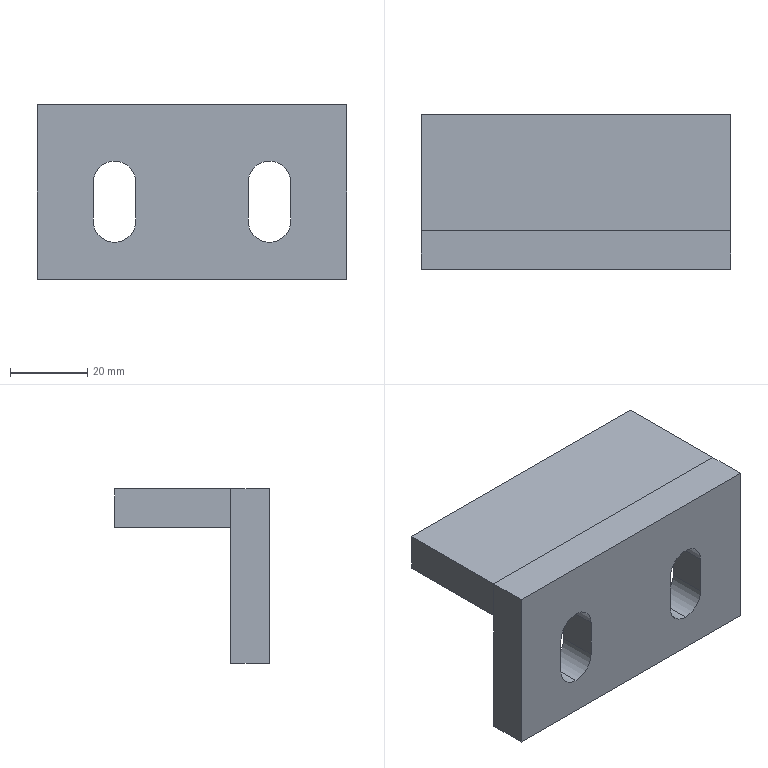Part | STEP file | BCC3 H11_2B | 2 solids | 22 faces | box 80 x 40 x 45 mm | volume 55899 mm3 | plane 16 | cylinder 6 | commonest cylinder face diameters 11 x6